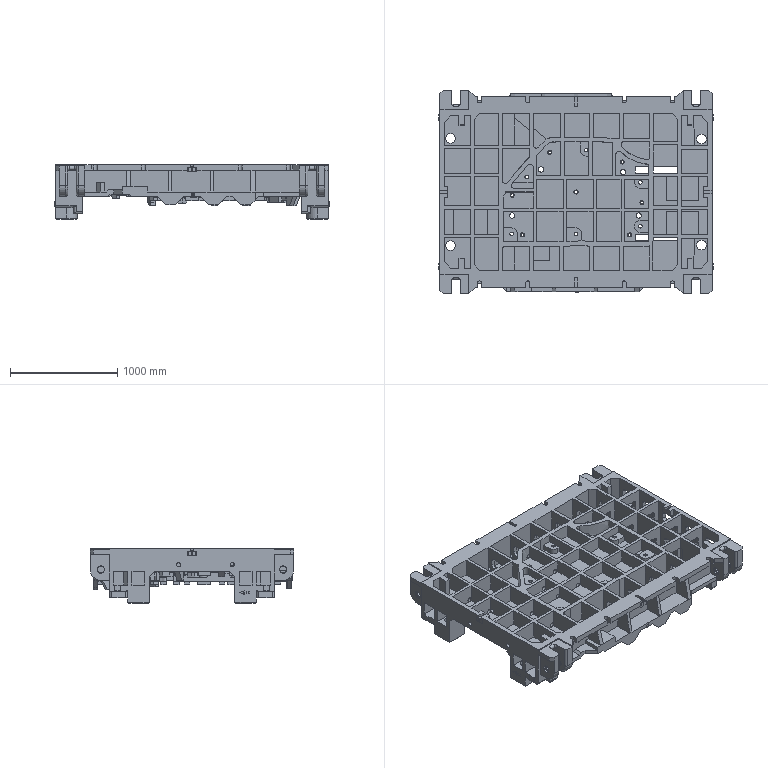Part | NX | features solid 2 | 1 solid | 2057 faces | box 2560 x 1900 x 510 mm | volume 529519437 mm3 | plane 1643 | cylinder 358 | spline 40 | torus 16 | commonest cylinder face diameters 60 x108 40 x83 68 x48 64 x16 80 x15 30 x14